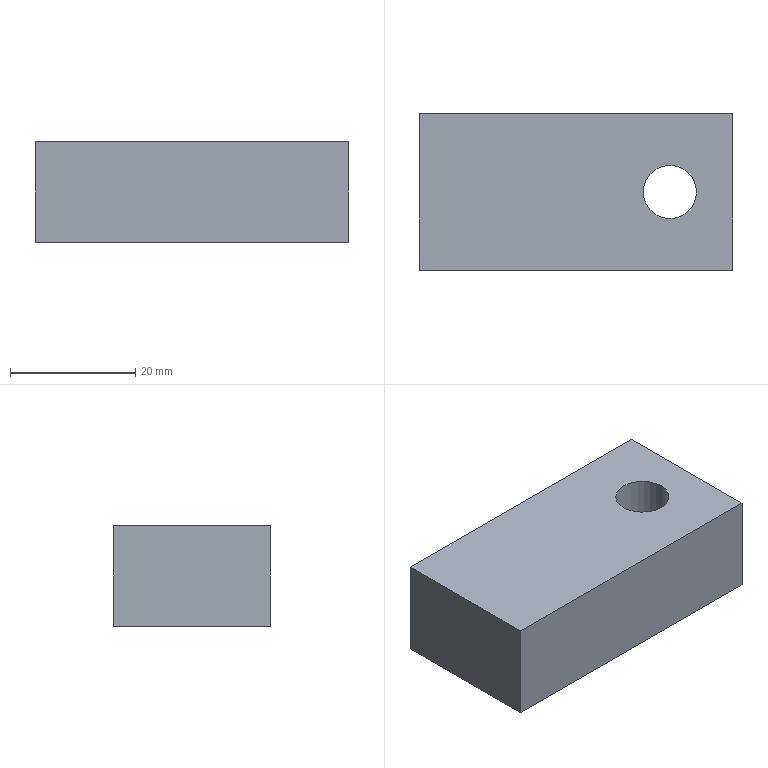Part | SolidWorks | features FlatPattern 1, HoleWzd 1, SMBaseFlange 1, SheetMetal 1 | 1 solid | 8 faces | box 50 x 25 x 16 mm | volume 19092 mm3 | plane 6 | cylinder 2 | commonest cylinder face diameters 8.5 x2
STEP:
#1=CARTESIAN_POINT('',(35.75,-12.5,-16.));
#2=VERTEX_POINT('',#1);
#3=CARTESIAN_POINT('',(44.25,-12.5,-16.));
#4=VERTEX_POINT('',#3);
#5=CARTESIAN_POINT('',(40.,-12.5,-16.));
#6=DIRECTION('',(0.,0.,1.));
#7=DIRECTION('',(1.,0.,0.));
#8=AXIS2_PLACEMENT_3D('',#5,#6,#7);
#9=CIRCLE('',#8,4.25);
#10=EDGE_CURVE('',#2,#4,#9,.T.);
#11=ORIENTED_EDGE('',*,*,#10,.F.);
#12=CARTESIAN_POINT('',(35.75,-12.5,0.));
#13=VERTEX_POINT('',#12);
#14=CARTESIAN_POINT('',(35.75,-12.5,0.));
#15=DIRECTION('',(0.,0.,1.));
#16=VECTOR('',#15,1000.);
#17=LINE('',#14,#16);
#18=EDGE_CURVE('',#2,#13,#17,.T.);
#19=ORIENTED_EDGE('',*,*,#18,.T.);
#20=CARTESIAN_POINT('',(44.25,-12.5,0.));
#21=VERTEX_POINT('',#20);
#22=CARTESIAN_POINT('',(40.,-12.5,0.));
#23=DIRECTION('',(0.,0.,1.));
#24=DIRECTION('',(1.,0.,0.));
#25=AXIS2_PLACEMENT_3D('',#22,#23,#24);
#26=CIRCLE('',#25,4.25);
#27=EDGE_CURVE('',#13,#21,#26,.T.);
#28=ORIENTED_EDGE('',*,*,#27,.T.);
#29=CARTESIAN_POINT('',(44.25,-12.5,0.));
#30=DIRECTION('',(0.,0.,1.));
#31=VECTOR('',#30,1000.);
#32=LINE('',#29,#31);
#33=EDGE_CURVE('',#4,#21,#32,.T.);
#34=ORIENTED_EDGE('',*,*,#33,.F.);
#35=EDGE_LOOP('',(#11,#19,#28,#34));
#36=FACE_OUTER_BOUND('',#35,.T.);
#37=CARTESIAN_POINT('',(40.,-12.5,0.));
#38=DIRECTION('',(0.,0.,1.));
#39=DIRECTION('',(1.,0.,0.));
#40=AXIS2_PLACEMENT_3D('',#37,#38,#39);
#41=CYLINDRICAL_SURFACE('',#40,4.25);
#42=ADVANCED_FACE('',(#36),#41,.F.);
#43=CARTESIAN_POINT('',(0.,0.,0.));
#44=VERTEX_POINT('',#43);
#45=CARTESIAN_POINT('',(0.,-25.,0.));
#46=VERTEX_POINT('',#45);
#47=CARTESIAN_POINT('',(0.,0.,0.));
#48=DIRECTION('',(0.,-1.,0.));
#49=VECTOR('',#48,1000.);
#50=LINE('',#47,#49);
#51=EDGE_CURVE('',#44,#46,#50,.T.);
#52=ORIENTED_EDGE('',*,*,#51,.F.);
#53=CARTESIAN_POINT('',(0.,0.,-16.));
#54=VERTEX_POINT('',#53);
#55=CARTESIAN_POINT('',(0.,0.,-16.));
#56=DIRECTION('',(0.,0.,1.));
#57=VECTOR('',#56,1000.);
#58=LINE('',#55,#57);
#59=EDGE_CURVE('',#54,#44,#58,.T.);
#60=ORIENTED_EDGE('',*,*,#59,.F.);
#61=CARTESIAN_POINT('',(0.,-25.,-16.));
#62=VERTEX_POINT('',#61);
#63=CARTESIAN_POINT('',(0.,0.,-16.));
#64=DIRECTION('',(0.,-1.,0.));
#65=VECTOR('',#64,1000.);
#66=LINE('',#63,#65);
#67=EDGE_CURVE('',#54,#62,#66,.T.);
#68=ORIENTED_EDGE('',*,*,#67,.T.);
#69=CARTESIAN_POINT('',(0.,-25.,-16.));
#70=DIRECTION('',(0.,0.,1.));
#71=VECTOR('',#70,1000.);
#72=LINE('',#69,#71);
#73=EDGE_CURVE('',#62,#46,#72,.T.);
#74=ORIENTED_EDGE('',*,*,#73,.T.);
#75=EDGE_LOOP('',(#52,#60,#68,#74));
#76=FACE_OUTER_BOUND('',#75,.T.);
#77=CARTESIAN_POINT('',(0.,0.,-16.));
#78=DIRECTION('',(-1.,0.,0.));
#79=DIRECTION('',(0.,-1.,0.));
#80=AXIS2_PLACEMENT_3D('',#77,#78,#79);
#81=PLANE('',#80);
#82=ADVANCED_FACE('',(#76),#81,.T.);
#83=CARTESIAN_POINT('',(50.,0.,0.));
#84=VERTEX_POINT('',#83);
#85=CARTESIAN_POINT('',(0.,0.,0.));
#86=DIRECTION('',(-1.,0.,0.));
#87=VECTOR('',#86,1000.);
#88=LINE('',#85,#87);
#89=EDGE_CURVE('',#84,#44,#88,.T.);
#90=ORIENTED_EDGE('',*,*,#89,.F.);
#91=CARTESIAN_POINT('',(50.,0.,-16.));
#92=VERTEX_POINT('',#91);
#93=CARTESIAN_POINT('',(50.,0.,-16.));
#94=DIRECTION('',(0.,0.,1.));
#95=VECTOR('',#94,1000.);
#96=LINE('',#93,#95);
#97=EDGE_CURVE('',#92,#84,#96,.T.);
#98=ORIENTED_EDGE('',*,*,#97,.F.);
#99=CARTESIAN_POINT('',(0.,0.,-16.));
#100=DIRECTION('',(-1.,0.,0.));
#101=VECTOR('',#100,1000.);
#102=LINE('',#99,#101);
#103=EDGE_CURVE('',#92,#54,#102,.T.);
#104=ORIENTED_EDGE('',*,*,#103,.T.);
#105=ORIENTED_EDGE('',*,*,#59,.T.);
#106=EDGE_LOOP('',(#90,#98,#104,#105));
#107=FACE_OUTER_BOUND('',#106,.T.);
#108=CARTESIAN_POINT('',(0.,0.,-16.));
#109=DIRECTION('',(0.,1.,0.));
#110=DIRECTION('',(0.,0.,1.));
#111=AXIS2_PLACEMENT_3D('',#108,#109,#110);
#112=PLANE('',#111);
#113=ADVANCED_FACE('',(#107),#112,.T.);
#114=CARTESIAN_POINT('',(50.,-25.,0.));
#115=VERTEX_POINT('',#114);
#116=CARTESIAN_POINT('',(50.,0.,0.));
#117=DIRECTION('',(0.,1.,0.));
#118=VECTOR('',#117,1000.);
#119=LINE('',#116,#118);
#120=EDGE_CURVE('',#115,#84,#119,.T.);
#121=ORIENTED_EDGE('',*,*,#120,.F.);
#122=CARTESIAN_POINT('',(50.,-25.,-16.));
#123=VERTEX_POINT('',#122);
#124=CARTESIAN_POINT('',(50.,-25.,-16.));
#125=DIRECTION('',(0.,0.,1.));
#126=VECTOR('',#125,1000.);
#127=LINE('',#124,#126);
#128=EDGE_CURVE('',#123,#115,#127,.T.);
#129=ORIENTED_EDGE('',*,*,#128,.F.);
#130=CARTESIAN_POINT('',(50.,0.,-16.));
#131=DIRECTION('',(0.,1.,0.));
#132=VECTOR('',#131,1000.);
#133=LINE('',#130,#132);
#134=EDGE_CURVE('',#123,#92,#133,.T.);
#135=ORIENTED_EDGE('',*,*,#134,.T.);
#136=ORIENTED_EDGE('',*,*,#97,.T.);
#137=EDGE_LOOP('',(#121,#129,#135,#136));
#138=FACE_OUTER_BOUND('',#137,.T.);
#139=CARTESIAN_POINT('',(50.,0.,-16.));
#140=DIRECTION('',(1.,0.,0.));
#141=DIRECTION('',(0.,0.,-1.));
#142=AXIS2_PLACEMENT_3D('',#139,#140,#141);
#143=PLANE('',#142);
#144=ADVANCED_FACE('',(#138),#143,.T.);
#145=CARTESIAN_POINT('',(0.,-25.,0.));
#146=DIRECTION('',(1.,0.,0.));
#147=VECTOR('',#146,1000.);
#148=LINE('',#145,#147);
#149=EDGE_CURVE('',#46,#115,#148,.T.);
#150=ORIENTED_EDGE('',*,*,#149,.F.);
#151=ORIENTED_EDGE('',*,*,#73,.F.);
#152=CARTESIAN_POINT('',(0.,-25.,-16.));
#153=DIRECTION('',(1.,0.,0.));
#154=VECTOR('',#153,1000.);
#155=LINE('',#152,#154);
#156=EDGE_CURVE('',#62,#123,#155,.T.);
#157=ORIENTED_EDGE('',*,*,#156,.T.);
#158=ORIENTED_EDGE('',*,*,#128,.T.);
#159=EDGE_LOOP('',(#150,#151,#157,#158));
#160=FACE_OUTER_BOUND('',#159,.T.);
#161=CARTESIAN_POINT('',(0.,-25.,-16.));
#162=DIRECTION('',(0.,-1.,0.));
#163=DIRECTION('',(0.,0.,-1.));
#164=AXIS2_PLACEMENT_3D('',#161,#162,#163);
#165=PLANE('',#164);
#166=ADVANCED_FACE('',(#160),#165,.T.);
#167=CARTESIAN_POINT('',(40.,-12.5,-16.));
#168=DIRECTION('',(0.,0.,1.));
#169=DIRECTION('',(1.,0.,0.));
#170=AXIS2_PLACEMENT_3D('',#167,#168,#169);
#171=CIRCLE('',#170,4.25);
#172=EDGE_CURVE('',#4,#2,#171,.T.);
#173=ORIENTED_EDGE('',*,*,#172,.T.);
#174=ORIENTED_EDGE('',*,*,#10,.T.);
#175=EDGE_LOOP('',(#173,#174));
#176=FACE_BOUND('',#175,.T.);
#177=ORIENTED_EDGE('',*,*,#67,.F.);
#178=ORIENTED_EDGE('',*,*,#103,.F.);
#179=ORIENTED_EDGE('',*,*,#134,.F.);
#180=ORIENTED_EDGE('',*,*,#156,.F.);
#181=EDGE_LOOP('',(#177,#178,#179,#180));
#182=FACE_OUTER_BOUND('',#181,.T.);
#183=CARTESIAN_POINT('',(0.,0.,-16.));
#184=DIRECTION('',(0.,0.,1.));
#185=DIRECTION('',(1.,0.,0.));
#186=AXIS2_PLACEMENT_3D('',#183,#184,#185);
#187=PLANE('',#186);
#188=ADVANCED_FACE('',(#176,#182),#187,.F.);
#189=CARTESIAN_POINT('',(40.,-12.5,0.));
#190=DIRECTION('',(0.,0.,1.));
#191=DIRECTION('',(1.,0.,0.));
#192=AXIS2_PLACEMENT_3D('',#189,#190,#191);
#193=CIRCLE('',#192,4.25);
#194=EDGE_CURVE('',#21,#13,#193,.T.);
#195=ORIENTED_EDGE('',*,*,#194,.F.);
#196=ORIENTED_EDGE('',*,*,#27,.F.);
#197=EDGE_LOOP('',(#195,#196));
#198=FACE_BOUND('',#197,.T.);
#199=ORIENTED_EDGE('',*,*,#51,.T.);
#200=ORIENTED_EDGE('',*,*,#149,.T.);
#201=ORIENTED_EDGE('',*,*,#120,.T.);
#202=ORIENTED_EDGE('',*,*,#89,.T.);
#203=EDGE_LOOP('',(#199,#200,#201,#202));
#204=FACE_OUTER_BOUND('',#203,.T.);
#205=CARTESIAN_POINT('',(0.,0.,0.));
#206=DIRECTION('',(0.,0.,1.));
#207=DIRECTION('',(1.,0.,0.));
#208=AXIS2_PLACEMENT_3D('',#205,#206,#207);
#209=PLANE('',#208);
#210=ADVANCED_FACE('',(#198,#204),#209,.T.);
#211=ORIENTED_EDGE('',*,*,#18,.F.);
#212=ORIENTED_EDGE('',*,*,#172,.F.);
#213=ORIENTED_EDGE('',*,*,#33,.T.);
#214=ORIENTED_EDGE('',*,*,#194,.T.);
#215=EDGE_LOOP('',(#211,#212,#213,#214));
#216=FACE_OUTER_BOUND('',#215,.T.);
#217=CARTESIAN_POINT('',(40.,-12.5,0.));
#218=DIRECTION('',(0.,0.,1.));
#219=DIRECTION('',(1.,0.,0.));
#220=AXIS2_PLACEMENT_3D('',#217,#218,#219);
#221=CYLINDRICAL_SURFACE('',#220,4.25);
#222=ADVANCED_FACE('',(#216),#221,.F.);
#223=CLOSED_SHELL('',(#42,#82,#113,#144,#166,#188,#210,#222));
#224=MANIFOLD_SOLID_BREP('',#223);
#225=CARTESIAN_POINT('',(0.,0.,0.));
#226=DIRECTION('',(0.,0.,1.));
#227=DIRECTION('',(1.,0.,0.));
#228=AXIS2_PLACEMENT_3D('',#225,#226,#227);
#229=(LENGTH_UNIT()NAMED_UNIT(*)SI_UNIT(.MILLI.,.METRE.));
#230=UNCERTAINTY_MEASURE_WITH_UNIT(LENGTH_MEASURE(0.00001),#229,'','');
#231=(NAMED_UNIT(*)PLANE_ANGLE_UNIT()SI_UNIT($,.RADIAN.));
#232=(NAMED_UNIT(*)SI_UNIT($,.STERADIAN.)SOLID_ANGLE_UNIT());
#233=(GEOMETRIC_REPRESENTATION_CONTEXT(3)GLOBAL_UNCERTAINTY_ASSIGNED_CONTEXT((#230))GLOBAL_UNIT_ASSIGNED_CONTEXT((#229,#231,#232))REPRESENTATION_CONTEXT('',''));
#234=ADVANCED_BREP_SHAPE_REPRESENTATION('',(#224,#228),#233);